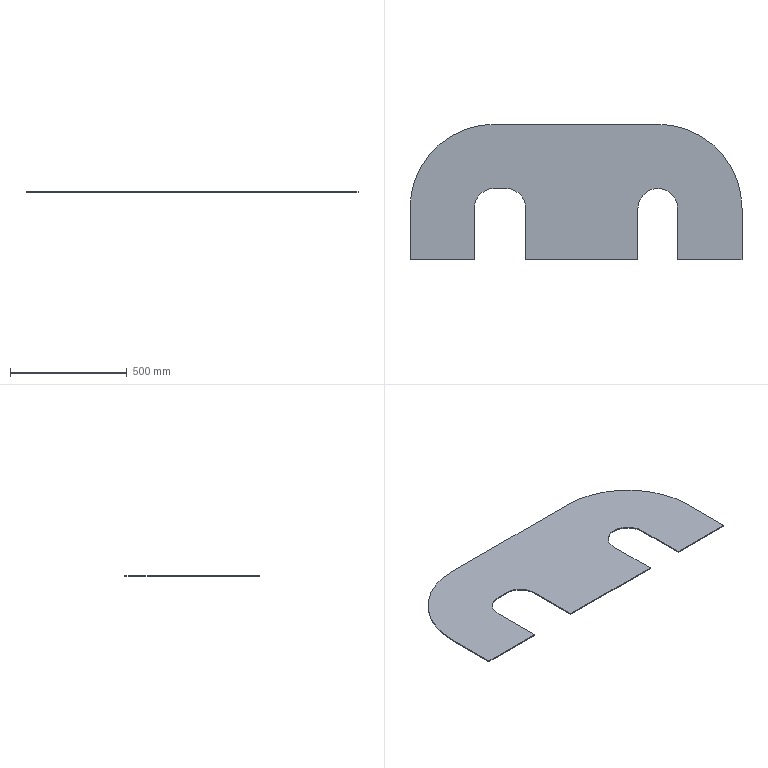Part | NX | features BREP 1 | 1 solid | 18 faces | box 1420 x 580 x 4 mm | volume 2620909 mm3 | plane 13 | cylinder 5 | commonest cylinder face diameters 170 x3 720 x2
STEP:
#1=CARTESIAN_POINT('',(-785.,0.,0.));
#2=VERTEX_POINT('',#1);
#3=CARTESIAN_POINT('',(-700.,85.,0.));
#4=VERTEX_POINT('',#3);
#5=CARTESIAN_POINT('',(-700.,0.,0.));
#6=DIRECTION('',(0.,0.,-1.));
#7=DIRECTION('',(1.,0.,0.));
#8=AXIS2_PLACEMENT_3D('',#5,#6,#7);
#9=CIRCLE('',#8,85.);
#10=EDGE_CURVE('',#2,#4,#9,.T.);
#11=ORIENTED_EDGE('',*,*,#10,.T.);
#12=CARTESIAN_POINT('',(-700.,85.,4.));
#13=VERTEX_POINT('',#12);
#14=CARTESIAN_POINT('',(-700.,85.,4.));
#15=DIRECTION('',(0.,0.,-1.));
#16=VECTOR('',#15,1000.);
#17=LINE('',#14,#16);
#18=EDGE_CURVE('',#13,#4,#17,.T.);
#19=ORIENTED_EDGE('',*,*,#18,.F.);
#20=CARTESIAN_POINT('',(-785.,0.,4.));
#21=VERTEX_POINT('',#20);
#22=CARTESIAN_POINT('',(-700.,0.,4.));
#23=DIRECTION('',(0.,0.,-1.));
#24=DIRECTION('',(1.,0.,0.));
#25=AXIS2_PLACEMENT_3D('',#22,#23,#24);
#26=CIRCLE('',#25,85.);
#27=EDGE_CURVE('',#21,#13,#26,.T.);
#28=ORIENTED_EDGE('',*,*,#27,.F.);
#29=CARTESIAN_POINT('',(-785.,0.,4.));
#30=DIRECTION('',(0.,0.,-1.));
#31=VECTOR('',#30,1000.);
#32=LINE('',#29,#31);
#33=EDGE_CURVE('',#21,#2,#32,.T.);
#34=ORIENTED_EDGE('',*,*,#33,.T.);
#35=EDGE_LOOP('',(#11,#19,#28,#34));
#36=FACE_BOUND('',#35,.T.);
#37=CARTESIAN_POINT('',(-700.,0.,4.));
#38=DIRECTION('',(0.,0.,-1.));
#39=DIRECTION('',(1.,0.,0.));
#40=AXIS2_PLACEMENT_3D('',#37,#38,#39);
#41=CYLINDRICAL_SURFACE('',#40,85.);
#42=ADVANCED_FACE('',(#36),#41,.F.);
#43=CARTESIAN_POINT('',(-650.,85.,0.));
#44=VERTEX_POINT('',#43);
#45=CARTESIAN_POINT('',(-700.,85.,0.));
#46=DIRECTION('',(1.,0.,0.));
#47=VECTOR('',#46,1000.);
#48=LINE('',#45,#47);
#49=EDGE_CURVE('',#4,#44,#48,.T.);
#50=ORIENTED_EDGE('',*,*,#49,.T.);
#51=CARTESIAN_POINT('',(-650.,85.,4.));
#52=VERTEX_POINT('',#51);
#53=CARTESIAN_POINT('',(-650.,85.,4.));
#54=DIRECTION('',(0.,0.,-1.));
#55=VECTOR('',#54,1000.);
#56=LINE('',#53,#55);
#57=EDGE_CURVE('',#52,#44,#56,.T.);
#58=ORIENTED_EDGE('',*,*,#57,.F.);
#59=CARTESIAN_POINT('',(-700.,85.,4.));
#60=DIRECTION('',(1.,0.,0.));
#61=VECTOR('',#60,1000.);
#62=LINE('',#59,#61);
#63=EDGE_CURVE('',#13,#52,#62,.T.);
#64=ORIENTED_EDGE('',*,*,#63,.F.);
#65=ORIENTED_EDGE('',*,*,#18,.T.);
#66=EDGE_LOOP('',(#50,#58,#64,#65));
#67=FACE_BOUND('',#66,.T.);
#68=CARTESIAN_POINT('',(-700.,85.,4.));
#69=DIRECTION('',(0.,1.,0.));
#70=DIRECTION('',(1.,0.,0.));
#71=AXIS2_PLACEMENT_3D('',#68,#69,#70);
#72=PLANE('',#71);
#73=ADVANCED_FACE('',(#67),#72,.F.);
#74=CARTESIAN_POINT('',(-565.,0.,0.));
#75=VERTEX_POINT('',#74);
#76=CARTESIAN_POINT('',(-650.,0.,0.));
#77=DIRECTION('',(0.,0.,-1.));
#78=DIRECTION('',(1.,0.,0.));
#79=AXIS2_PLACEMENT_3D('',#76,#77,#78);
#80=CIRCLE('',#79,85.);
#81=EDGE_CURVE('',#44,#75,#80,.T.);
#82=ORIENTED_EDGE('',*,*,#81,.T.);
#83=CARTESIAN_POINT('',(-565.,0.,4.));
#84=VERTEX_POINT('',#83);
#85=CARTESIAN_POINT('',(-565.,0.,4.));
#86=DIRECTION('',(0.,0.,-1.));
#87=VECTOR('',#86,1000.);
#88=LINE('',#85,#87);
#89=EDGE_CURVE('',#84,#75,#88,.T.);
#90=ORIENTED_EDGE('',*,*,#89,.F.);
#91=CARTESIAN_POINT('',(-650.,0.,4.));
#92=DIRECTION('',(0.,0.,-1.));
#93=DIRECTION('',(1.,0.,0.));
#94=AXIS2_PLACEMENT_3D('',#91,#92,#93);
#95=CIRCLE('',#94,85.);
#96=EDGE_CURVE('',#52,#84,#95,.T.);
#97=ORIENTED_EDGE('',*,*,#96,.F.);
#98=ORIENTED_EDGE('',*,*,#57,.T.);
#99=EDGE_LOOP('',(#82,#90,#97,#98));
#100=FACE_BOUND('',#99,.T.);
#101=CARTESIAN_POINT('',(-650.,0.,4.));
#102=DIRECTION('',(0.,0.,-1.));
#103=DIRECTION('',(1.,0.,0.));
#104=AXIS2_PLACEMENT_3D('',#101,#102,#103);
#105=CYLINDRICAL_SURFACE('',#104,85.);
#106=ADVANCED_FACE('',(#100),#105,.F.);
#107=CARTESIAN_POINT('',(-565.,-220.,0.));
#108=VERTEX_POINT('',#107);
#109=CARTESIAN_POINT('',(-565.,0.,0.));
#110=DIRECTION('',(0.,-1.,0.));
#111=VECTOR('',#110,1000.);
#112=LINE('',#109,#111);
#113=EDGE_CURVE('',#75,#108,#112,.T.);
#114=ORIENTED_EDGE('',*,*,#113,.T.);
#115=CARTESIAN_POINT('',(-565.,-220.,4.));
#116=VERTEX_POINT('',#115);
#117=CARTESIAN_POINT('',(-565.,-220.,4.));
#118=DIRECTION('',(0.,0.,-1.));
#119=VECTOR('',#118,1000.);
#120=LINE('',#117,#119);
#121=EDGE_CURVE('',#116,#108,#120,.T.);
#122=ORIENTED_EDGE('',*,*,#121,.F.);
#123=CARTESIAN_POINT('',(-565.,0.,4.));
#124=DIRECTION('',(0.,-1.,0.));
#125=VECTOR('',#124,1000.);
#126=LINE('',#123,#125);
#127=EDGE_CURVE('',#84,#116,#126,.T.);
#128=ORIENTED_EDGE('',*,*,#127,.F.);
#129=ORIENTED_EDGE('',*,*,#89,.T.);
#130=EDGE_LOOP('',(#114,#122,#128,#129));
#131=FACE_BOUND('',#130,.T.);
#132=CARTESIAN_POINT('',(-565.,0.,4.));
#133=DIRECTION('',(1.,0.,0.));
#134=DIRECTION('',(0.,0.,1.));
#135=AXIS2_PLACEMENT_3D('',#132,#133,#134);
#136=PLANE('',#135);
#137=ADVANCED_FACE('',(#131),#136,.F.);
#138=CARTESIAN_POINT('',(-85.,-220.,0.));
#139=VERTEX_POINT('',#138);
#140=CARTESIAN_POINT('',(-565.,-220.,0.));
#141=DIRECTION('',(1.,0.,0.));
#142=VECTOR('',#141,1000.);
#143=LINE('',#140,#142);
#144=EDGE_CURVE('',#108,#139,#143,.T.);
#145=ORIENTED_EDGE('',*,*,#144,.T.);
#146=CARTESIAN_POINT('',(-85.,-220.,4.));
#147=VERTEX_POINT('',#146);
#148=CARTESIAN_POINT('',(-85.,-220.,4.));
#149=DIRECTION('',(0.,0.,-1.));
#150=VECTOR('',#149,1000.);
#151=LINE('',#148,#150);
#152=EDGE_CURVE('',#147,#139,#151,.T.);
#153=ORIENTED_EDGE('',*,*,#152,.F.);
#154=CARTESIAN_POINT('',(-565.,-220.,4.));
#155=DIRECTION('',(1.,0.,0.));
#156=VECTOR('',#155,1000.);
#157=LINE('',#154,#156);
#158=EDGE_CURVE('',#116,#147,#157,.T.);
#159=ORIENTED_EDGE('',*,*,#158,.F.);
#160=ORIENTED_EDGE('',*,*,#121,.T.);
#161=EDGE_LOOP('',(#145,#153,#159,#160));
#162=FACE_BOUND('',#161,.T.);
#163=CARTESIAN_POINT('',(-565.,-220.,4.));
#164=DIRECTION('',(0.,1.,0.));
#165=DIRECTION('',(0.,0.,-1.));
#166=AXIS2_PLACEMENT_3D('',#163,#164,#165);
#167=PLANE('',#166);
#168=ADVANCED_FACE('',(#162),#167,.F.);
#169=CARTESIAN_POINT('',(-85.,0.,0.));
#170=VERTEX_POINT('',#169);
#171=CARTESIAN_POINT('',(-85.,0.,0.));
#172=DIRECTION('',(0.,1.,0.));
#173=VECTOR('',#172,1000.);
#174=LINE('',#171,#173);
#175=EDGE_CURVE('',#139,#170,#174,.T.);
#176=ORIENTED_EDGE('',*,*,#175,.T.);
#177=CARTESIAN_POINT('',(-85.,0.,4.));
#178=VERTEX_POINT('',#177);
#179=CARTESIAN_POINT('',(-85.,0.,4.));
#180=DIRECTION('',(0.,0.,-1.));
#181=VECTOR('',#180,1000.);
#182=LINE('',#179,#181);
#183=EDGE_CURVE('',#178,#170,#182,.T.);
#184=ORIENTED_EDGE('',*,*,#183,.F.);
#185=CARTESIAN_POINT('',(-85.,0.,4.));
#186=DIRECTION('',(0.,1.,0.));
#187=VECTOR('',#186,1000.);
#188=LINE('',#185,#187);
#189=EDGE_CURVE('',#147,#178,#188,.T.);
#190=ORIENTED_EDGE('',*,*,#189,.F.);
#191=ORIENTED_EDGE('',*,*,#152,.T.);
#192=EDGE_LOOP('',(#176,#184,#190,#191));
#193=FACE_BOUND('',#192,.T.);
#194=CARTESIAN_POINT('',(-85.,0.,4.));
#195=DIRECTION('',(-1.,0.,0.));
#196=DIRECTION('',(0.,1.,0.));
#197=AXIS2_PLACEMENT_3D('',#194,#195,#196);
#198=PLANE('',#197);
#199=ADVANCED_FACE('',(#193),#198,.F.);
#200=CARTESIAN_POINT('',(85.,0.,0.));
#201=VERTEX_POINT('',#200);
#202=CARTESIAN_POINT('',(0.,0.,0.));
#203=DIRECTION('',(0.,0.,-1.));
#204=DIRECTION('',(1.,0.,0.));
#205=AXIS2_PLACEMENT_3D('',#202,#203,#204);
#206=CIRCLE('',#205,85.);
#207=EDGE_CURVE('',#170,#201,#206,.T.);
#208=ORIENTED_EDGE('',*,*,#207,.T.);
#209=CARTESIAN_POINT('',(85.,0.,4.));
#210=VERTEX_POINT('',#209);
#211=CARTESIAN_POINT('',(85.,0.,4.));
#212=DIRECTION('',(0.,0.,-1.));
#213=VECTOR('',#212,1000.);
#214=LINE('',#211,#213);
#215=EDGE_CURVE('',#210,#201,#214,.T.);
#216=ORIENTED_EDGE('',*,*,#215,.F.);
#217=CARTESIAN_POINT('',(0.,0.,4.));
#218=DIRECTION('',(0.,0.,-1.));
#219=DIRECTION('',(1.,0.,0.));
#220=AXIS2_PLACEMENT_3D('',#217,#218,#219);
#221=CIRCLE('',#220,85.);
#222=EDGE_CURVE('',#178,#210,#221,.T.);
#223=ORIENTED_EDGE('',*,*,#222,.F.);
#224=ORIENTED_EDGE('',*,*,#183,.T.);
#225=EDGE_LOOP('',(#208,#216,#223,#224));
#226=FACE_BOUND('',#225,.T.);
#227=CARTESIAN_POINT('',(0.,0.,4.));
#228=DIRECTION('',(0.,0.,-1.));
#229=DIRECTION('',(1.,0.,0.));
#230=AXIS2_PLACEMENT_3D('',#227,#228,#229);
#231=CYLINDRICAL_SURFACE('',#230,85.);
#232=ADVANCED_FACE('',(#226),#231,.F.);
#233=CARTESIAN_POINT('',(85.,-220.,0.));
#234=VERTEX_POINT('',#233);
#235=CARTESIAN_POINT('',(85.,0.,0.));
#236=DIRECTION('',(0.,-1.,0.));
#237=VECTOR('',#236,1000.);
#238=LINE('',#235,#237);
#239=EDGE_CURVE('',#201,#234,#238,.T.);
#240=ORIENTED_EDGE('',*,*,#239,.T.);
#241=CARTESIAN_POINT('',(85.,-220.,4.));
#242=VERTEX_POINT('',#241);
#243=CARTESIAN_POINT('',(85.,-220.,4.));
#244=DIRECTION('',(0.,0.,-1.));
#245=VECTOR('',#244,1000.);
#246=LINE('',#243,#245);
#247=EDGE_CURVE('',#242,#234,#246,.T.);
#248=ORIENTED_EDGE('',*,*,#247,.F.);
#249=CARTESIAN_POINT('',(85.,0.,4.));
#250=DIRECTION('',(0.,-1.,0.));
#251=VECTOR('',#250,1000.);
#252=LINE('',#249,#251);
#253=EDGE_CURVE('',#210,#242,#252,.T.);
#254=ORIENTED_EDGE('',*,*,#253,.F.);
#255=ORIENTED_EDGE('',*,*,#215,.T.);
#256=EDGE_LOOP('',(#240,#248,#254,#255));
#257=FACE_BOUND('',#256,.T.);
#258=CARTESIAN_POINT('',(85.,0.,4.));
#259=DIRECTION('',(1.,0.,0.));
#260=DIRECTION('',(0.,-1.,0.));
#261=AXIS2_PLACEMENT_3D('',#258,#259,#260);
#262=PLANE('',#261);
#263=ADVANCED_FACE('',(#257),#262,.F.);
#264=CARTESIAN_POINT('',(360.,-220.,0.));
#265=VERTEX_POINT('',#264);
#266=CARTESIAN_POINT('',(85.,-220.,0.));
#267=DIRECTION('',(1.,0.,0.));
#268=VECTOR('',#267,1000.);
#269=LINE('',#266,#268);
#270=EDGE_CURVE('',#234,#265,#269,.T.);
#271=ORIENTED_EDGE('',*,*,#270,.T.);
#272=CARTESIAN_POINT('',(360.,-220.,4.));
#273=VERTEX_POINT('',#272);
#274=CARTESIAN_POINT('',(360.,-220.,4.));
#275=DIRECTION('',(0.,0.,-1.));
#276=VECTOR('',#275,1000.);
#277=LINE('',#274,#276);
#278=EDGE_CURVE('',#273,#265,#277,.T.);
#279=ORIENTED_EDGE('',*,*,#278,.F.);
#280=CARTESIAN_POINT('',(85.,-220.,4.));
#281=DIRECTION('',(1.,0.,0.));
#282=VECTOR('',#281,1000.);
#283=LINE('',#280,#282);
#284=EDGE_CURVE('',#242,#273,#283,.T.);
#285=ORIENTED_EDGE('',*,*,#284,.F.);
#286=ORIENTED_EDGE('',*,*,#247,.T.);
#287=EDGE_LOOP('',(#271,#279,#285,#286));
#288=FACE_BOUND('',#287,.T.);
#289=CARTESIAN_POINT('',(85.,-220.,4.));
#290=DIRECTION('',(0.,1.,0.));
#291=DIRECTION('',(0.,0.,-1.));
#292=AXIS2_PLACEMENT_3D('',#289,#290,#291);
#293=PLANE('',#292);
#294=ADVANCED_FACE('',(#288),#293,.F.);
#295=CARTESIAN_POINT('',(360.,0.,0.));
#296=VERTEX_POINT('',#295);
#297=CARTESIAN_POINT('',(360.,-220.,0.));
#298=DIRECTION('',(0.,1.,0.));
#299=VECTOR('',#298,1000.);
#300=LINE('',#297,#299);
#301=EDGE_CURVE('',#265,#296,#300,.T.);
#302=ORIENTED_EDGE('',*,*,#301,.T.);
#303=CARTESIAN_POINT('',(360.,0.,4.));
#304=VERTEX_POINT('',#303);
#305=CARTESIAN_POINT('',(360.,0.,4.));
#306=DIRECTION('',(0.,0.,-1.));
#307=VECTOR('',#306,1000.);
#308=LINE('',#305,#307);
#309=EDGE_CURVE('',#304,#296,#308,.T.);
#310=ORIENTED_EDGE('',*,*,#309,.F.);
#311=CARTESIAN_POINT('',(360.,-220.,4.));
#312=DIRECTION('',(0.,1.,0.));
#313=VECTOR('',#312,1000.);
#314=LINE('',#311,#313);
#315=EDGE_CURVE('',#273,#304,#314,.T.);
#316=ORIENTED_EDGE('',*,*,#315,.F.);
#317=ORIENTED_EDGE('',*,*,#278,.T.);
#318=EDGE_LOOP('',(#302,#310,#316,#317));
#319=FACE_BOUND('',#318,.T.);
#320=CARTESIAN_POINT('',(360.,-220.,4.));
#321=DIRECTION('',(-1.,0.,0.));
#322=DIRECTION('',(0.,0.,-1.));
#323=AXIS2_PLACEMENT_3D('',#320,#321,#322);
#324=PLANE('',#323);
#325=ADVANCED_FACE('',(#319),#324,.F.);
#326=CARTESIAN_POINT('',(0.,360.,0.));
#327=VERTEX_POINT('',#326);
#328=CARTESIAN_POINT('',(0.,0.,0.));
#329=DIRECTION('',(0.,0.,1.));
#330=DIRECTION('',(1.,0.,0.));
#331=AXIS2_PLACEMENT_3D('',#328,#329,#330);
#332=CIRCLE('',#331,360.);
#333=EDGE_CURVE('',#296,#327,#332,.T.);
#334=ORIENTED_EDGE('',*,*,#333,.T.);
#335=CARTESIAN_POINT('',(0.,360.,4.));
#336=VERTEX_POINT('',#335);
#337=CARTESIAN_POINT('',(0.,360.,4.));
#338=DIRECTION('',(0.,0.,-1.));
#339=VECTOR('',#338,1000.);
#340=LINE('',#337,#339);
#341=EDGE_CURVE('',#336,#327,#340,.T.);
#342=ORIENTED_EDGE('',*,*,#341,.F.);
#343=CARTESIAN_POINT('',(0.,0.,4.));
#344=DIRECTION('',(0.,0.,1.));
#345=DIRECTION('',(1.,0.,0.));
#346=AXIS2_PLACEMENT_3D('',#343,#344,#345);
#347=CIRCLE('',#346,360.);
#348=EDGE_CURVE('',#304,#336,#347,.T.);
#349=ORIENTED_EDGE('',*,*,#348,.F.);
#350=ORIENTED_EDGE('',*,*,#309,.T.);
#351=EDGE_LOOP('',(#334,#342,#349,#350));
#352=FACE_BOUND('',#351,.T.);
#353=CARTESIAN_POINT('',(0.,0.,4.));
#354=DIRECTION('',(0.,0.,-1.));
#355=DIRECTION('',(1.,0.,0.));
#356=AXIS2_PLACEMENT_3D('',#353,#354,#355);
#357=CYLINDRICAL_SURFACE('',#356,360.);
#358=ADVANCED_FACE('',(#352),#357,.T.);
#359=CARTESIAN_POINT('',(-700.,360.,0.));
#360=VERTEX_POINT('',#359);
#361=CARTESIAN_POINT('',(-700.,360.,0.));
#362=DIRECTION('',(-1.,0.,0.));
#363=VECTOR('',#362,1000.);
#364=LINE('',#361,#363);
#365=EDGE_CURVE('',#327,#360,#364,.T.);
#366=ORIENTED_EDGE('',*,*,#365,.T.);
#367=CARTESIAN_POINT('',(-700.,360.,4.));
#368=VERTEX_POINT('',#367);
#369=CARTESIAN_POINT('',(-700.,360.,4.));
#370=DIRECTION('',(0.,0.,-1.));
#371=VECTOR('',#370,1000.);
#372=LINE('',#369,#371);
#373=EDGE_CURVE('',#368,#360,#372,.T.);
#374=ORIENTED_EDGE('',*,*,#373,.F.);
#375=CARTESIAN_POINT('',(-700.,360.,4.));
#376=DIRECTION('',(-1.,0.,0.));
#377=VECTOR('',#376,1000.);
#378=LINE('',#375,#377);
#379=EDGE_CURVE('',#336,#368,#378,.T.);
#380=ORIENTED_EDGE('',*,*,#379,.F.);
#381=ORIENTED_EDGE('',*,*,#341,.T.);
#382=EDGE_LOOP('',(#366,#374,#380,#381));
#383=FACE_BOUND('',#382,.T.);
#384=CARTESIAN_POINT('',(-700.,360.,4.));
#385=DIRECTION('',(0.,-1.,0.));
#386=DIRECTION('',(0.,0.,1.));
#387=AXIS2_PLACEMENT_3D('',#384,#385,#386);
#388=PLANE('',#387);
#389=ADVANCED_FACE('',(#383),#388,.F.);
#390=CARTESIAN_POINT('',(-1060.,0.,0.));
#391=VERTEX_POINT('',#390);
#392=CARTESIAN_POINT('',(-700.,0.,0.));
#393=DIRECTION('',(0.,0.,1.));
#394=DIRECTION('',(1.,0.,0.));
#395=AXIS2_PLACEMENT_3D('',#392,#393,#394);
#396=CIRCLE('',#395,360.);
#397=EDGE_CURVE('',#360,#391,#396,.T.);
#398=ORIENTED_EDGE('',*,*,#397,.T.);
#399=CARTESIAN_POINT('',(-1060.,0.,4.));
#400=VERTEX_POINT('',#399);
#401=CARTESIAN_POINT('',(-1060.,0.,4.));
#402=DIRECTION('',(0.,0.,-1.));
#403=VECTOR('',#402,1000.);
#404=LINE('',#401,#403);
#405=EDGE_CURVE('',#400,#391,#404,.T.);
#406=ORIENTED_EDGE('',*,*,#405,.F.);
#407=CARTESIAN_POINT('',(-700.,0.,4.));
#408=DIRECTION('',(0.,0.,1.));
#409=DIRECTION('',(1.,0.,0.));
#410=AXIS2_PLACEMENT_3D('',#407,#408,#409);
#411=CIRCLE('',#410,360.);
#412=EDGE_CURVE('',#368,#400,#411,.T.);
#413=ORIENTED_EDGE('',*,*,#412,.F.);
#414=ORIENTED_EDGE('',*,*,#373,.T.);
#415=EDGE_LOOP('',(#398,#406,#413,#414));
#416=FACE_BOUND('',#415,.T.);
#417=CARTESIAN_POINT('',(-700.,0.,4.));
#418=DIRECTION('',(0.,0.,-1.));
#419=DIRECTION('',(1.,0.,0.));
#420=AXIS2_PLACEMENT_3D('',#417,#418,#419);
#421=CYLINDRICAL_SURFACE('',#420,360.);
#422=ADVANCED_FACE('',(#416),#421,.T.);
#423=CARTESIAN_POINT('',(-1060.,-220.,0.));
#424=VERTEX_POINT('',#423);
#425=CARTESIAN_POINT('',(-1060.,0.,0.));
#426=DIRECTION('',(0.,-1.,0.));
#427=VECTOR('',#426,1000.);
#428=LINE('',#425,#427);
#429=EDGE_CURVE('',#391,#424,#428,.T.);
#430=ORIENTED_EDGE('',*,*,#429,.T.);
#431=CARTESIAN_POINT('',(-1060.,-220.,4.));
#432=VERTEX_POINT('',#431);
#433=CARTESIAN_POINT('',(-1060.,-220.,4.));
#434=DIRECTION('',(0.,0.,-1.));
#435=VECTOR('',#434,1000.);
#436=LINE('',#433,#435);
#437=EDGE_CURVE('',#432,#424,#436,.T.);
#438=ORIENTED_EDGE('',*,*,#437,.F.);
#439=CARTESIAN_POINT('',(-1060.,0.,4.));
#440=DIRECTION('',(0.,-1.,0.));
#441=VECTOR('',#440,1000.);
#442=LINE('',#439,#441);
#443=EDGE_CURVE('',#400,#432,#442,.T.);
#444=ORIENTED_EDGE('',*,*,#443,.F.);
#445=ORIENTED_EDGE('',*,*,#405,.T.);
#446=EDGE_LOOP('',(#430,#438,#444,#445));
#447=FACE_BOUND('',#446,.T.);
#448=CARTESIAN_POINT('',(-1060.,0.,4.));
#449=DIRECTION('',(1.,0.,0.));
#450=DIRECTION('',(0.,0.,1.));
#451=AXIS2_PLACEMENT_3D('',#448,#449,#450);
#452=PLANE('',#451);
#453=ADVANCED_FACE('',(#447),#452,.F.);
#454=CARTESIAN_POINT('',(-785.,-220.,0.));
#455=VERTEX_POINT('',#454);
#456=CARTESIAN_POINT('',(-785.,-220.,0.));
#457=DIRECTION('',(1.,0.,0.));
#458=VECTOR('',#457,1000.);
#459=LINE('',#456,#458);
#460=EDGE_CURVE('',#424,#455,#459,.T.);
#461=ORIENTED_EDGE('',*,*,#460,.T.);
#462=CARTESIAN_POINT('',(-785.,-220.,4.));
#463=VERTEX_POINT('',#462);
#464=CARTESIAN_POINT('',(-785.,-220.,4.));
#465=DIRECTION('',(0.,0.,-1.));
#466=VECTOR('',#465,1000.);
#467=LINE('',#464,#466);
#468=EDGE_CURVE('',#463,#455,#467,.T.);
#469=ORIENTED_EDGE('',*,*,#468,.F.);
#470=CARTESIAN_POINT('',(-785.,-220.,4.));
#471=DIRECTION('',(1.,0.,0.));
#472=VECTOR('',#471,1000.);
#473=LINE('',#470,#472);
#474=EDGE_CURVE('',#432,#463,#473,.T.);
#475=ORIENTED_EDGE('',*,*,#474,.F.);
#476=ORIENTED_EDGE('',*,*,#437,.T.);
#477=EDGE_LOOP('',(#461,#469,#475,#476));
#478=FACE_BOUND('',#477,.T.);
#479=CARTESIAN_POINT('',(-785.,-220.,4.));
#480=DIRECTION('',(0.,1.,0.));
#481=DIRECTION('',(0.,0.,-1.));
#482=AXIS2_PLACEMENT_3D('',#479,#480,#481);
#483=PLANE('',#482);
#484=ADVANCED_FACE('',(#478),#483,.F.);
#485=CARTESIAN_POINT('',(-785.,0.,0.));
#486=DIRECTION('',(0.,1.,0.));
#487=VECTOR('',#486,1000.);
#488=LINE('',#485,#487);
#489=EDGE_CURVE('',#455,#2,#488,.T.);
#490=ORIENTED_EDGE('',*,*,#489,.T.);
#491=ORIENTED_EDGE('',*,*,#33,.F.);
#492=CARTESIAN_POINT('',(-785.,0.,4.));
#493=DIRECTION('',(0.,1.,0.));
#494=VECTOR('',#493,1000.);
#495=LINE('',#492,#494);
#496=EDGE_CURVE('',#463,#21,#495,.T.);
#497=ORIENTED_EDGE('',*,*,#496,.F.);
#498=ORIENTED_EDGE('',*,*,#468,.T.);
#499=EDGE_LOOP('',(#490,#491,#497,#498));
#500=FACE_BOUND('',#499,.T.);
#501=CARTESIAN_POINT('',(-785.,0.,4.));
#502=DIRECTION('',(-1.,0.,0.));
#503=DIRECTION('',(0.,0.,-1.));
#504=AXIS2_PLACEMENT_3D('',#501,#502,#503);
#505=PLANE('',#504);
#506=ADVANCED_FACE('',(#500),#505,.F.);
#507=ORIENTED_EDGE('',*,*,#27,.T.);
#508=ORIENTED_EDGE('',*,*,#63,.T.);
#509=ORIENTED_EDGE('',*,*,#96,.T.);
#510=ORIENTED_EDGE('',*,*,#127,.T.);
#511=ORIENTED_EDGE('',*,*,#158,.T.);
#512=ORIENTED_EDGE('',*,*,#189,.T.);
#513=ORIENTED_EDGE('',*,*,#222,.T.);
#514=ORIENTED_EDGE('',*,*,#253,.T.);
#515=ORIENTED_EDGE('',*,*,#284,.T.);
#516=ORIENTED_EDGE('',*,*,#315,.T.);
#517=ORIENTED_EDGE('',*,*,#348,.T.);
#518=ORIENTED_EDGE('',*,*,#379,.T.);
#519=ORIENTED_EDGE('',*,*,#412,.T.);
#520=ORIENTED_EDGE('',*,*,#443,.T.);
#521=ORIENTED_EDGE('',*,*,#474,.T.);
#522=ORIENTED_EDGE('',*,*,#496,.T.);
#523=EDGE_LOOP('',(#507,#508,#509,#510,#511,#512,#513,#514,#515,#516,#517,#518,#519,#520,#521,#522));
#524=FACE_BOUND('',#523,.T.);
#525=CARTESIAN_POINT('',(-700.,0.,4.));
#526=DIRECTION('',(0.,0.,1.));
#527=DIRECTION('',(-1.,0.,0.));
#528=AXIS2_PLACEMENT_3D('',#525,#526,#527);
#529=PLANE('',#528);
#530=ADVANCED_FACE('',(#524),#529,.T.);
#531=ORIENTED_EDGE('',*,*,#10,.F.);
#532=ORIENTED_EDGE('',*,*,#489,.F.);
#533=ORIENTED_EDGE('',*,*,#460,.F.);
#534=ORIENTED_EDGE('',*,*,#429,.F.);
#535=ORIENTED_EDGE('',*,*,#397,.F.);
#536=ORIENTED_EDGE('',*,*,#365,.F.);
#537=ORIENTED_EDGE('',*,*,#333,.F.);
#538=ORIENTED_EDGE('',*,*,#301,.F.);
#539=ORIENTED_EDGE('',*,*,#270,.F.);
#540=ORIENTED_EDGE('',*,*,#239,.F.);
#541=ORIENTED_EDGE('',*,*,#207,.F.);
#542=ORIENTED_EDGE('',*,*,#175,.F.);
#543=ORIENTED_EDGE('',*,*,#144,.F.);
#544=ORIENTED_EDGE('',*,*,#113,.F.);
#545=ORIENTED_EDGE('',*,*,#81,.F.);
#546=ORIENTED_EDGE('',*,*,#49,.F.);
#547=EDGE_LOOP('',(#531,#532,#533,#534,#535,#536,#537,#538,#539,#540,#541,#542,#543,#544,#545,#546));
#548=FACE_BOUND('',#547,.T.);
#549=CARTESIAN_POINT('',(-700.,0.,0.));
#550=DIRECTION('',(0.,0.,1.));
#551=DIRECTION('',(-1.,0.,0.));
#552=AXIS2_PLACEMENT_3D('',#549,#550,#551);
#553=PLANE('',#552);
#554=ADVANCED_FACE('',(#548),#553,.F.);
#555=CLOSED_SHELL('',(#42,#73,#106,#137,#168,#199,#232,#263,#294,#325,#358,#389,#422,#453,#484,#506,#530,#554));
#556=MANIFOLD_SOLID_BREP('',#555);
#557=(LENGTH_UNIT()NAMED_UNIT(*)SI_UNIT(.MILLI.,.METRE.));
#558=UNCERTAINTY_MEASURE_WITH_UNIT(LENGTH_MEASURE(0.00001),#557,'','');
#559=(NAMED_UNIT(*)PLANE_ANGLE_UNIT()SI_UNIT($,.RADIAN.));
#560=(NAMED_UNIT(*)SI_UNIT($,.STERADIAN.)SOLID_ANGLE_UNIT());
#561=(GEOMETRIC_REPRESENTATION_CONTEXT(3)GLOBAL_UNCERTAINTY_ASSIGNED_CONTEXT((#558))GLOBAL_UNIT_ASSIGNED_CONTEXT((#557,#559,#560))REPRESENTATION_CONTEXT('',''));
#562=ADVANCED_BREP_SHAPE_REPRESENTATION('',(#556),#561);